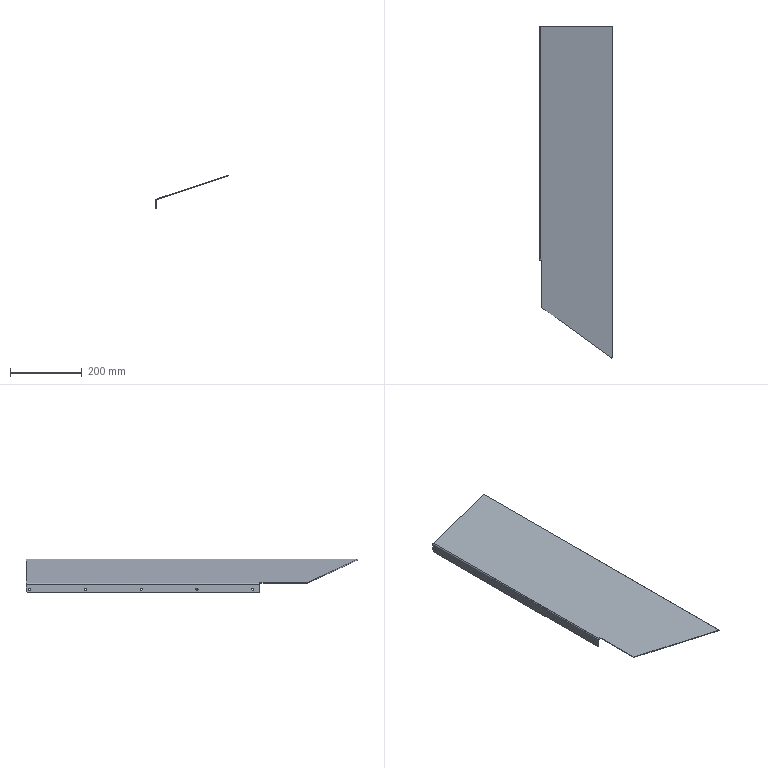Part | NX | features solid 2 | 1 solid | 25 faces | box 203 x 924.5 x 93.897 mm | volume 393378 mm3 | cylinder 14 | plane 11 | commonest cylinder face diameters 6 x10 4 x2 8 x1 20 x1
STEP:
#1=CARTESIAN_POINT('',(2192.368,-654.75,255.897));
#2=VERTEX_POINT('',#1);
#3=CARTESIAN_POINT('',(2190.47,-652.75,255.265));
#4=VERTEX_POINT('',#3);
#5=CARTESIAN_POINT('',(2190.47,-654.75,255.265));
#6=DIRECTION('',(-0.3162,0.,0.9487));
#7=DIRECTION('',(-0.9487,0.,-0.3162));
#8=AXIS2_PLACEMENT_3D('',#5,#6,#7);
#9=CIRCLE('',#8,2.);
#10=EDGE_CURVE('',#2,#4,#9,.T.);
#11=ORIENTED_EDGE('',*,*,#10,.F.);
#12=CARTESIAN_POINT('',(2193.,-654.75,254.));
#13=VERTEX_POINT('',#12);
#14=CARTESIAN_POINT('',(2193.,-654.75,254.));
#15=DIRECTION('',(-0.3162,0.,0.9487));
#16=VECTOR('',#15,1000.);
#17=LINE('',#14,#16);
#18=EDGE_CURVE('',#13,#2,#17,.T.);
#19=ORIENTED_EDGE('',*,*,#18,.F.);
#20=CARTESIAN_POINT('',(2191.103,-652.75,253.368));
#21=VERTEX_POINT('',#20);
#22=CARTESIAN_POINT('',(2191.103,-654.75,253.368));
#23=DIRECTION('',(0.3162,0.,-0.9487));
#24=DIRECTION('',(-0.9487,0.,-0.3162));
#25=AXIS2_PLACEMENT_3D('',#22,#23,#24);
#26=CIRCLE('',#25,2.);
#27=EDGE_CURVE('',#21,#13,#26,.T.);
#28=ORIENTED_EDGE('',*,*,#27,.F.);
#29=CARTESIAN_POINT('',(2191.735,-652.75,251.47));
#30=DIRECTION('',(0.3162,0.,-0.9487));
#31=VECTOR('',#30,1000.);
#32=LINE('',#29,#31);
#33=EDGE_CURVE('',#4,#21,#32,.T.);
#34=ORIENTED_EDGE('',*,*,#33,.F.);
#35=EDGE_LOOP('',(#11,#19,#28,#34));
#36=FACE_BOUND('',#35,.T.);
#37=CARTESIAN_POINT('',(2191.735,-654.75,251.47));
#38=DIRECTION('',(0.3162,0.,-0.9487));
#39=DIRECTION('',(0.9487,0.,0.3162));
#40=AXIS2_PLACEMENT_3D('',#37,#38,#39);
#41=CYLINDRICAL_SURFACE('',#40,2.);
#42=ADVANCED_FACE('',(#36),#41,.T.);
#43=CARTESIAN_POINT('',(1990.,-652.75,172.));
#44=VERTEX_POINT('',#43);
#45=CARTESIAN_POINT('',(1990.,-662.75,162.));
#46=VERTEX_POINT('',#45);
#47=CARTESIAN_POINT('',(1990.,-662.75,172.));
#48=DIRECTION('',(-1.,0.,0.));
#49=DIRECTION('',(0.,0.,-1.));
#50=AXIS2_PLACEMENT_3D('',#47,#48,#49);
#51=CIRCLE('',#50,10.);
#52=EDGE_CURVE('',#44,#46,#51,.T.);
#53=ORIENTED_EDGE('',*,*,#52,.F.);
#54=CARTESIAN_POINT('',(1992.,-652.75,172.));
#55=VERTEX_POINT('',#54);
#56=CARTESIAN_POINT('',(1994.,-652.75,172.));
#57=DIRECTION('',(-1.,0.,0.));
#58=VECTOR('',#57,1000.);
#59=LINE('',#56,#58);
#60=EDGE_CURVE('',#55,#44,#59,.T.);
#61=ORIENTED_EDGE('',*,*,#60,.F.);
#62=CARTESIAN_POINT('',(1992.,-662.75,162.));
#63=VERTEX_POINT('',#62);
#64=CARTESIAN_POINT('',(1992.,-662.75,172.));
#65=DIRECTION('',(1.,0.,0.));
#66=DIRECTION('',(0.,0.,-1.));
#67=AXIS2_PLACEMENT_3D('',#64,#65,#66);
#68=CIRCLE('',#67,10.);
#69=EDGE_CURVE('',#63,#55,#68,.T.);
#70=ORIENTED_EDGE('',*,*,#69,.F.);
#71=CARTESIAN_POINT('',(1992.,-662.75,162.));
#72=DIRECTION('',(1.,0.,0.));
#73=VECTOR('',#72,1000.);
#74=LINE('',#71,#73);
#75=EDGE_CURVE('',#46,#63,#74,.T.);
#76=ORIENTED_EDGE('',*,*,#75,.F.);
#77=EDGE_LOOP('',(#53,#61,#70,#76));
#78=FACE_BOUND('',#77,.T.);
#79=CARTESIAN_POINT('',(1992.,-662.75,172.));
#80=DIRECTION('',(-1.,0.,0.));
#81=DIRECTION('',(0.,-1.,0.));
#82=AXIS2_PLACEMENT_3D('',#79,#80,#81);
#83=CYLINDRICAL_SURFACE('',#82,10.);
#84=ADVANCED_FACE('',(#78),#83,.T.);
#85=CARTESIAN_POINT('',(1992.,-1284.25,175.));
#86=VERTEX_POINT('',#85);
#87=CARTESIAN_POINT('',(1990.,-1284.25,175.));
#88=VERTEX_POINT('',#87);
#89=CARTESIAN_POINT('',(2941.171,-1284.25,175.));
#90=DIRECTION('',(-1.,0.,0.));
#91=VECTOR('',#90,1000.);
#92=LINE('',#89,#91);
#93=EDGE_CURVE('',#86,#88,#92,.T.);
#94=ORIENTED_EDGE('',*,*,#93,.F.);
#95=CARTESIAN_POINT('',(1992.,-1284.25,169.));
#96=VERTEX_POINT('',#95);
#97=CARTESIAN_POINT('',(1992.,-1284.25,172.));
#98=DIRECTION('',(-1.,0.,0.));
#99=DIRECTION('',(0.,0.,-1.));
#100=AXIS2_PLACEMENT_3D('',#97,#98,#99);
#101=CIRCLE('',#100,3.);
#102=EDGE_CURVE('',#96,#86,#101,.T.);
#103=ORIENTED_EDGE('',*,*,#102,.F.);
#104=CARTESIAN_POINT('',(1990.,-1284.25,169.));
#105=VERTEX_POINT('',#104);
#106=CARTESIAN_POINT('',(2941.171,-1284.25,169.));
#107=DIRECTION('',(-1.,0.,0.));
#108=VECTOR('',#107,1000.);
#109=LINE('',#106,#108);
#110=EDGE_CURVE('',#105,#96,#109,.F.);
#111=ORIENTED_EDGE('',*,*,#110,.F.);
#112=CARTESIAN_POINT('',(1990.,-1284.25,172.));
#113=DIRECTION('',(-1.,0.,0.));
#114=DIRECTION('',(0.,-1.,0.));
#115=AXIS2_PLACEMENT_3D('',#112,#113,#114);
#116=CIRCLE('',#115,3.);
#117=EDGE_CURVE('',#105,#88,#116,.T.);
#118=ORIENTED_EDGE('',*,*,#117,.T.);
#119=EDGE_LOOP('',(#94,#103,#111,#118));
#120=FACE_BOUND('',#119,.T.);
#121=CARTESIAN_POINT('',(2941.171,-1284.25,172.));
#122=DIRECTION('',(-1.,0.,0.));
#123=DIRECTION('',(0.,0.,-1.));
#124=AXIS2_PLACEMENT_3D('',#121,#122,#123);
#125=CYLINDRICAL_SURFACE('',#124,3.);
#126=ADVANCED_FACE('',(#120),#125,.F.);
#127=CARTESIAN_POINT('',(1990.,-1128.875,175.));
#128=VERTEX_POINT('',#127);
#129=CARTESIAN_POINT('',(1992.,-1128.875,175.));
#130=VERTEX_POINT('',#129);
#131=CARTESIAN_POINT('',(2941.171,-1128.875,175.));
#132=DIRECTION('',(-1.,0.,0.));
#133=VECTOR('',#132,1000.);
#134=LINE('',#131,#133);
#135=EDGE_CURVE('',#128,#130,#134,.F.);
#136=ORIENTED_EDGE('',*,*,#135,.T.);
#137=CARTESIAN_POINT('',(1992.,-1128.875,169.));
#138=VERTEX_POINT('',#137);
#139=CARTESIAN_POINT('',(1992.,-1128.875,172.));
#140=DIRECTION('',(-1.,0.,0.));
#141=DIRECTION('',(0.,0.,-1.));
#142=AXIS2_PLACEMENT_3D('',#139,#140,#141);
#143=CIRCLE('',#142,3.);
#144=EDGE_CURVE('',#138,#130,#143,.T.);
#145=ORIENTED_EDGE('',*,*,#144,.F.);
#146=CARTESIAN_POINT('',(1990.,-1128.875,169.));
#147=VERTEX_POINT('',#146);
#148=CARTESIAN_POINT('',(2941.171,-1128.875,169.));
#149=DIRECTION('',(-1.,0.,0.));
#150=VECTOR('',#149,1000.);
#151=LINE('',#148,#150);
#152=EDGE_CURVE('',#138,#147,#151,.T.);
#153=ORIENTED_EDGE('',*,*,#152,.T.);
#154=CARTESIAN_POINT('',(1990.,-1128.875,172.));
#155=DIRECTION('',(-1.,0.,0.));
#156=DIRECTION('',(0.,-1.,0.));
#157=AXIS2_PLACEMENT_3D('',#154,#155,#156);
#158=CIRCLE('',#157,3.);
#159=EDGE_CURVE('',#147,#128,#158,.T.);
#160=ORIENTED_EDGE('',*,*,#159,.T.);
#161=EDGE_LOOP('',(#136,#145,#153,#160));
#162=FACE_BOUND('',#161,.T.);
#163=CARTESIAN_POINT('',(2941.171,-1128.875,172.));
#164=DIRECTION('',(-1.,0.,0.));
#165=DIRECTION('',(0.,0.,-1.));
#166=AXIS2_PLACEMENT_3D('',#163,#164,#165);
#167=CYLINDRICAL_SURFACE('',#166,3.);
#168=ADVANCED_FACE('',(#162),#167,.F.);
#169=CARTESIAN_POINT('',(1992.,-973.5,175.));
#170=VERTEX_POINT('',#169);
#171=CARTESIAN_POINT('',(1990.,-973.5,175.));
#172=VERTEX_POINT('',#171);
#173=CARTESIAN_POINT('',(2941.171,-973.5,175.));
#174=DIRECTION('',(-1.,0.,0.));
#175=VECTOR('',#174,1000.);
#176=LINE('',#173,#175);
#177=EDGE_CURVE('',#170,#172,#176,.T.);
#178=ORIENTED_EDGE('',*,*,#177,.F.);
#179=CARTESIAN_POINT('',(1992.,-973.5,169.));
#180=VERTEX_POINT('',#179);
#181=CARTESIAN_POINT('',(1992.,-973.5,172.));
#182=DIRECTION('',(-1.,0.,0.));
#183=DIRECTION('',(0.,0.,-1.));
#184=AXIS2_PLACEMENT_3D('',#181,#182,#183);
#185=CIRCLE('',#184,3.);
#186=EDGE_CURVE('',#180,#170,#185,.T.);
#187=ORIENTED_EDGE('',*,*,#186,.F.);
#188=CARTESIAN_POINT('',(1990.,-973.5,169.));
#189=VERTEX_POINT('',#188);
#190=CARTESIAN_POINT('',(2941.171,-973.5,169.));
#191=DIRECTION('',(-1.,0.,0.));
#192=VECTOR('',#191,1000.);
#193=LINE('',#190,#192);
#194=EDGE_CURVE('',#189,#180,#193,.F.);
#195=ORIENTED_EDGE('',*,*,#194,.F.);
#196=CARTESIAN_POINT('',(1990.,-973.5,172.));
#197=DIRECTION('',(-1.,0.,0.));
#198=DIRECTION('',(0.,-1.,0.));
#199=AXIS2_PLACEMENT_3D('',#196,#197,#198);
#200=CIRCLE('',#199,3.);
#201=EDGE_CURVE('',#189,#172,#200,.T.);
#202=ORIENTED_EDGE('',*,*,#201,.T.);
#203=EDGE_LOOP('',(#178,#187,#195,#202));
#204=FACE_BOUND('',#203,.T.);
#205=CARTESIAN_POINT('',(2941.171,-973.5,172.));
#206=DIRECTION('',(-1.,0.,0.));
#207=DIRECTION('',(0.,0.,-1.));
#208=AXIS2_PLACEMENT_3D('',#205,#206,#207);
#209=CYLINDRICAL_SURFACE('',#208,3.);
#210=ADVANCED_FACE('',(#204),#209,.F.);
#211=CARTESIAN_POINT('',(1992.,-818.125,175.));
#212=VERTEX_POINT('',#211);
#213=CARTESIAN_POINT('',(1990.,-818.125,175.));
#214=VERTEX_POINT('',#213);
#215=CARTESIAN_POINT('',(2941.171,-818.125,175.));
#216=DIRECTION('',(-1.,0.,0.));
#217=VECTOR('',#216,1000.);
#218=LINE('',#215,#217);
#219=EDGE_CURVE('',#212,#214,#218,.T.);
#220=ORIENTED_EDGE('',*,*,#219,.F.);
#221=CARTESIAN_POINT('',(1992.,-818.125,169.));
#222=VERTEX_POINT('',#221);
#223=CARTESIAN_POINT('',(1992.,-818.125,172.));
#224=DIRECTION('',(-1.,0.,0.));
#225=DIRECTION('',(0.,0.,-1.));
#226=AXIS2_PLACEMENT_3D('',#223,#224,#225);
#227=CIRCLE('',#226,3.);
#228=EDGE_CURVE('',#222,#212,#227,.T.);
#229=ORIENTED_EDGE('',*,*,#228,.F.);
#230=CARTESIAN_POINT('',(1990.,-818.125,169.));
#231=VERTEX_POINT('',#230);
#232=CARTESIAN_POINT('',(2941.171,-818.125,169.));
#233=DIRECTION('',(-1.,0.,0.));
#234=VECTOR('',#233,1000.);
#235=LINE('',#232,#234);
#236=EDGE_CURVE('',#231,#222,#235,.F.);
#237=ORIENTED_EDGE('',*,*,#236,.F.);
#238=CARTESIAN_POINT('',(1990.,-818.125,172.));
#239=DIRECTION('',(-1.,0.,0.));
#240=DIRECTION('',(0.,-1.,0.));
#241=AXIS2_PLACEMENT_3D('',#238,#239,#240);
#242=CIRCLE('',#241,3.);
#243=EDGE_CURVE('',#231,#214,#242,.T.);
#244=ORIENTED_EDGE('',*,*,#243,.T.);
#245=EDGE_LOOP('',(#220,#229,#237,#244));
#246=FACE_BOUND('',#245,.T.);
#247=CARTESIAN_POINT('',(2941.171,-818.125,172.));
#248=DIRECTION('',(-1.,0.,0.));
#249=DIRECTION('',(0.,0.,-1.));
#250=AXIS2_PLACEMENT_3D('',#247,#248,#249);
#251=CYLINDRICAL_SURFACE('',#250,3.);
#252=ADVANCED_FACE('',(#246),#251,.F.);
#253=CARTESIAN_POINT('',(1992.,-662.75,175.));
#254=VERTEX_POINT('',#253);
#255=CARTESIAN_POINT('',(1990.,-662.75,175.));
#256=VERTEX_POINT('',#255);
#257=CARTESIAN_POINT('',(2941.171,-662.75,175.));
#258=DIRECTION('',(-1.,0.,0.));
#259=VECTOR('',#258,1000.);
#260=LINE('',#257,#259);
#261=EDGE_CURVE('',#254,#256,#260,.T.);
#262=ORIENTED_EDGE('',*,*,#261,.F.);
#263=CARTESIAN_POINT('',(1992.,-662.75,169.));
#264=VERTEX_POINT('',#263);
#265=CARTESIAN_POINT('',(1992.,-662.75,172.));
#266=DIRECTION('',(-1.,0.,0.));
#267=DIRECTION('',(0.,0.,-1.));
#268=AXIS2_PLACEMENT_3D('',#265,#266,#267);
#269=CIRCLE('',#268,3.);
#270=EDGE_CURVE('',#264,#254,#269,.T.);
#271=ORIENTED_EDGE('',*,*,#270,.F.);
#272=CARTESIAN_POINT('',(1990.,-662.75,169.));
#273=VERTEX_POINT('',#272);
#274=CARTESIAN_POINT('',(2941.171,-662.75,169.));
#275=DIRECTION('',(-1.,0.,0.));
#276=VECTOR('',#275,1000.);
#277=LINE('',#274,#276);
#278=EDGE_CURVE('',#273,#264,#277,.F.);
#279=ORIENTED_EDGE('',*,*,#278,.F.);
#280=CARTESIAN_POINT('',(1990.,-662.75,172.));
#281=DIRECTION('',(-1.,0.,0.));
#282=DIRECTION('',(0.,-1.,0.));
#283=AXIS2_PLACEMENT_3D('',#280,#281,#282);
#284=CIRCLE('',#283,3.);
#285=EDGE_CURVE('',#273,#256,#284,.T.);
#286=ORIENTED_EDGE('',*,*,#285,.T.);
#287=EDGE_LOOP('',(#262,#271,#279,#286));
#288=FACE_BOUND('',#287,.T.);
#289=CARTESIAN_POINT('',(2941.171,-662.75,172.));
#290=DIRECTION('',(-1.,0.,0.));
#291=DIRECTION('',(0.,0.,-1.));
#292=AXIS2_PLACEMENT_3D('',#289,#290,#291);
#293=CYLINDRICAL_SURFACE('',#292,3.);
#294=ADVANCED_FACE('',(#288),#293,.F.);
#295=CARTESIAN_POINT('',(1996.725,-1304.25,190.683));
#296=VERTEX_POINT('',#295);
#297=CARTESIAN_POINT('',(1992.735,-1304.25,189.353));
#298=VERTEX_POINT('',#297);
#299=CARTESIAN_POINT('',(1991.368,-1304.25,188.897));
#300=DIRECTION('',(-0.9487,0.,-0.3162));
#301=VECTOR('',#300,1000.);
#302=LINE('',#299,#301);
#303=EDGE_CURVE('',#296,#298,#302,.T.);
#304=ORIENTED_EDGE('',*,*,#303,.T.);
#305=CARTESIAN_POINT('',(1990.,-1304.25,185.558));
#306=VERTEX_POINT('',#305);
#307=CARTESIAN_POINT('',(1994.,-1304.25,185.558));
#308=DIRECTION('',(0.,-1.,0.));
#309=DIRECTION('',(0.,0.,1.));
#310=AXIS2_PLACEMENT_3D('',#307,#308,#309);
#311=CIRCLE('',#310,4.);
#312=EDGE_CURVE('',#298,#306,#311,.T.);
#313=ORIENTED_EDGE('',*,*,#312,.T.);
#314=CARTESIAN_POINT('',(1990.,-1304.25,162.));
#315=VERTEX_POINT('',#314);
#316=CARTESIAN_POINT('',(1990.,-1304.25,162.));
#317=DIRECTION('',(0.,0.,-1.));
#318=VECTOR('',#317,1000.);
#319=LINE('',#316,#318);
#320=EDGE_CURVE('',#306,#315,#319,.T.);
#321=ORIENTED_EDGE('',*,*,#320,.T.);
#322=CARTESIAN_POINT('',(1992.,-1304.25,162.));
#323=VERTEX_POINT('',#322);
#324=CARTESIAN_POINT('',(1992.,-1304.25,162.));
#325=DIRECTION('',(1.,0.,0.));
#326=VECTOR('',#325,1000.);
#327=LINE('',#324,#326);
#328=EDGE_CURVE('',#315,#323,#327,.T.);
#329=ORIENTED_EDGE('',*,*,#328,.T.);
#330=CARTESIAN_POINT('',(1992.,-1304.25,185.558));
#331=VERTEX_POINT('',#330);
#332=CARTESIAN_POINT('',(1992.,-1304.25,162.));
#333=DIRECTION('',(0.,0.,-1.));
#334=VECTOR('',#333,1000.);
#335=LINE('',#332,#334);
#336=EDGE_CURVE('',#331,#323,#335,.T.);
#337=ORIENTED_EDGE('',*,*,#336,.F.);
#338=CARTESIAN_POINT('',(1993.368,-1304.25,187.456));
#339=VERTEX_POINT('',#338);
#340=CARTESIAN_POINT('',(1994.,-1304.25,185.558));
#341=DIRECTION('',(0.,-1.,0.));
#342=DIRECTION('',(-1.,0.,0.));
#343=AXIS2_PLACEMENT_3D('',#340,#341,#342);
#344=CIRCLE('',#343,2.);
#345=EDGE_CURVE('',#339,#331,#344,.T.);
#346=ORIENTED_EDGE('',*,*,#345,.F.);
#347=CARTESIAN_POINT('',(1997.357,-1304.25,188.786));
#348=VERTEX_POINT('',#347);
#349=CARTESIAN_POINT('',(1992.,-1304.25,187.));
#350=DIRECTION('',(-0.9487,0.,-0.3162));
#351=VECTOR('',#350,1000.);
#352=LINE('',#349,#351);
#353=EDGE_CURVE('',#348,#339,#352,.T.);
#354=ORIENTED_EDGE('',*,*,#353,.F.);
#355=CARTESIAN_POINT('',(1997.357,-1304.25,188.786));
#356=DIRECTION('',(0.3162,0.,-0.9487));
#357=VECTOR('',#356,1000.);
#358=LINE('',#355,#357);
#359=EDGE_CURVE('',#296,#348,#358,.T.);
#360=ORIENTED_EDGE('',*,*,#359,.F.);
#361=EDGE_LOOP('',(#304,#313,#321,#329,#337,#346,#354,#360));
#362=FACE_BOUND('',#361,.T.);
#363=CARTESIAN_POINT('',(1992.,-1304.25,187.));
#364=DIRECTION('',(0.,1.,0.));
#365=DIRECTION('',(0.,0.,-1.));
#366=AXIS2_PLACEMENT_3D('',#363,#364,#365);
#367=PLANE('',#366);
#368=ADVANCED_FACE('',(#362),#367,.F.);
#369=CARTESIAN_POINT('',(1996.725,-1436.889,190.683));
#370=VERTEX_POINT('',#369);
#371=CARTESIAN_POINT('',(1997.357,-1436.889,188.786));
#372=VERTEX_POINT('',#371);
#373=CARTESIAN_POINT('',(1997.357,-1436.889,188.786));
#374=DIRECTION('',(0.3162,0.,-0.9487));
#375=VECTOR('',#374,1000.);
#376=LINE('',#373,#375);
#377=EDGE_CURVE('',#370,#372,#376,.T.);
#378=ORIENTED_EDGE('',*,*,#377,.T.);
#379=CARTESIAN_POINT('',(2191.103,-1577.25,253.368));
#380=VERTEX_POINT('',#379);
#381=CARTESIAN_POINT('',(2055.875,-1479.284,208.292));
#382=DIRECTION('',(-0.7818,0.5664,-0.2606));
#383=VECTOR('',#382,1000.);
#384=LINE('',#381,#383);
#385=EDGE_CURVE('',#380,#372,#384,.T.);
#386=ORIENTED_EDGE('',*,*,#385,.F.);
#387=CARTESIAN_POINT('',(2190.47,-1577.25,255.265));
#388=VERTEX_POINT('',#387);
#389=CARTESIAN_POINT('',(2191.103,-1577.25,253.368));
#390=DIRECTION('',(0.3162,0.,-0.9487));
#391=VECTOR('',#390,1000.);
#392=LINE('',#389,#391);
#393=EDGE_CURVE('',#388,#380,#392,.T.);
#394=ORIENTED_EDGE('',*,*,#393,.F.);
#395=CARTESIAN_POINT('',(2055.243,-1479.284,210.189));
#396=DIRECTION('',(-0.7818,0.5664,-0.2606));
#397=VECTOR('',#396,1000.);
#398=LINE('',#395,#397);
#399=EDGE_CURVE('',#388,#370,#398,.T.);
#400=ORIENTED_EDGE('',*,*,#399,.T.);
#401=EDGE_LOOP('',(#378,#386,#394,#400));
#402=FACE_BOUND('',#401,.T.);
#403=CARTESIAN_POINT('',(2055.875,-1479.284,208.292));
#404=DIRECTION('',(0.5373,0.8241,0.1791));
#405=DIRECTION('',(0.3162,0.,-0.9487));
#406=AXIS2_PLACEMENT_3D('',#403,#404,#405);
#407=PLANE('',#406);
#408=ADVANCED_FACE('',(#402),#407,.F.);
#409=ORIENTED_EDGE('',*,*,#359,.T.);
#410=CARTESIAN_POINT('',(1997.357,-1577.25,188.786));
#411=DIRECTION('',(0.,1.,0.));
#412=VECTOR('',#411,1000.);
#413=LINE('',#410,#412);
#414=EDGE_CURVE('',#372,#348,#413,.T.);
#415=ORIENTED_EDGE('',*,*,#414,.F.);
#416=ORIENTED_EDGE('',*,*,#377,.F.);
#417=CARTESIAN_POINT('',(1996.725,-1577.25,190.683));
#418=DIRECTION('',(0.,1.,0.));
#419=VECTOR('',#418,1000.);
#420=LINE('',#417,#419);
#421=EDGE_CURVE('',#370,#296,#420,.T.);
#422=ORIENTED_EDGE('',*,*,#421,.T.);
#423=EDGE_LOOP('',(#409,#415,#416,#422));
#424=FACE_BOUND('',#423,.T.);
#425=CARTESIAN_POINT('',(1997.357,-1577.25,188.786));
#426=DIRECTION('',(0.9487,0.,0.3162));
#427=DIRECTION('',(0.,-1.,0.));
#428=AXIS2_PLACEMENT_3D('',#425,#426,#427);
#429=PLANE('',#428);
#430=ADVANCED_FACE('',(#424),#429,.F.);
#431=CARTESIAN_POINT('',(2192.368,-1577.25,255.897));
#432=VERTEX_POINT('',#431);
#433=CARTESIAN_POINT('',(2192.368,-1577.25,255.897));
#434=DIRECTION('',(0.,1.,0.));
#435=VECTOR('',#434,1000.);
#436=LINE('',#433,#435);
#437=EDGE_CURVE('',#432,#2,#436,.T.);
#438=ORIENTED_EDGE('',*,*,#437,.T.);
#439=ORIENTED_EDGE('',*,*,#10,.T.);
#440=CARTESIAN_POINT('',(1992.735,-652.75,189.353));
#441=VERTEX_POINT('',#440);
#442=CARTESIAN_POINT('',(1991.368,-652.75,188.897));
#443=DIRECTION('',(0.9487,0.,0.3162));
#444=VECTOR('',#443,1000.);
#445=LINE('',#442,#444);
#446=EDGE_CURVE('',#441,#4,#445,.T.);
#447=ORIENTED_EDGE('',*,*,#446,.F.);
#448=CARTESIAN_POINT('',(1992.735,-1577.25,189.353));
#449=DIRECTION('',(0.,1.,0.));
#450=VECTOR('',#449,1000.);
#451=LINE('',#448,#450);
#452=EDGE_CURVE('',#298,#441,#451,.T.);
#453=ORIENTED_EDGE('',*,*,#452,.F.);
#454=ORIENTED_EDGE('',*,*,#303,.F.);
#455=ORIENTED_EDGE('',*,*,#421,.F.);
#456=ORIENTED_EDGE('',*,*,#399,.F.);
#457=CARTESIAN_POINT('',(1991.368,-1577.25,188.897));
#458=DIRECTION('',(0.9487,0.,0.3162));
#459=VECTOR('',#458,1000.);
#460=LINE('',#457,#459);
#461=EDGE_CURVE('',#388,#432,#460,.T.);
#462=ORIENTED_EDGE('',*,*,#461,.T.);
#463=EDGE_LOOP('',(#438,#439,#447,#453,#454,#455,#456,#462));
#464=FACE_BOUND('',#463,.T.);
#465=CARTESIAN_POINT('',(1991.368,-1577.25,188.897));
#466=DIRECTION('',(-0.3162,0.,0.9487));
#467=DIRECTION('',(0.,1.,0.));
#468=AXIS2_PLACEMENT_3D('',#465,#466,#467);
#469=PLANE('',#468);
#470=ADVANCED_FACE('',(#464),#469,.T.);
#471=ORIENTED_EDGE('',*,*,#312,.F.);
#472=ORIENTED_EDGE('',*,*,#452,.T.);
#473=CARTESIAN_POINT('',(1990.,-652.75,185.558));
#474=VERTEX_POINT('',#473);
#475=CARTESIAN_POINT('',(1994.,-652.75,185.558));
#476=DIRECTION('',(0.,1.,0.));
#477=DIRECTION('',(0.,0.,1.));
#478=AXIS2_PLACEMENT_3D('',#475,#476,#477);
#479=CIRCLE('',#478,4.);
#480=EDGE_CURVE('',#474,#441,#479,.T.);
#481=ORIENTED_EDGE('',*,*,#480,.F.);
#482=CARTESIAN_POINT('',(1990.,-1577.25,185.558));
#483=DIRECTION('',(0.,1.,0.));
#484=VECTOR('',#483,1000.);
#485=LINE('',#482,#484);
#486=EDGE_CURVE('',#306,#474,#485,.T.);
#487=ORIENTED_EDGE('',*,*,#486,.F.);
#488=EDGE_LOOP('',(#471,#472,#481,#487));
#489=FACE_BOUND('',#488,.T.);
#490=CARTESIAN_POINT('',(1994.,-1577.25,185.558));
#491=DIRECTION('',(0.,1.,0.));
#492=DIRECTION('',(0.,0.,1.));
#493=AXIS2_PLACEMENT_3D('',#490,#491,#492);
#494=CYLINDRICAL_SURFACE('',#493,4.);
#495=ADVANCED_FACE('',(#489),#494,.T.);
#496=ORIENTED_EDGE('',*,*,#285,.F.);
#497=CARTESIAN_POINT('',(1990.,-662.75,172.));
#498=DIRECTION('',(-1.,0.,0.));
#499=DIRECTION('',(0.,-1.,0.));
#500=AXIS2_PLACEMENT_3D('',#497,#498,#499);
#501=CIRCLE('',#500,3.);
#502=EDGE_CURVE('',#256,#273,#501,.T.);
#503=ORIENTED_EDGE('',*,*,#502,.F.);
#504=EDGE_LOOP('',(#496,#503));
#505=FACE_BOUND('',#504,.T.);
#506=ORIENTED_EDGE('',*,*,#243,.F.);
#507=CARTESIAN_POINT('',(1990.,-818.125,172.));
#508=DIRECTION('',(-1.,0.,0.));
#509=DIRECTION('',(0.,-1.,0.));
#510=AXIS2_PLACEMENT_3D('',#507,#508,#509);
#511=CIRCLE('',#510,3.);
#512=EDGE_CURVE('',#214,#231,#511,.T.);
#513=ORIENTED_EDGE('',*,*,#512,.F.);
#514=EDGE_LOOP('',(#506,#513));
#515=FACE_BOUND('',#514,.T.);
#516=ORIENTED_EDGE('',*,*,#201,.F.);
#517=CARTESIAN_POINT('',(1990.,-973.5,172.));
#518=DIRECTION('',(-1.,0.,0.));
#519=DIRECTION('',(0.,-1.,0.));
#520=AXIS2_PLACEMENT_3D('',#517,#518,#519);
#521=CIRCLE('',#520,3.);
#522=EDGE_CURVE('',#172,#189,#521,.T.);
#523=ORIENTED_EDGE('',*,*,#522,.F.);
#524=EDGE_LOOP('',(#516,#523));
#525=FACE_BOUND('',#524,.T.);
#526=ORIENTED_EDGE('',*,*,#159,.F.);
#527=CARTESIAN_POINT('',(1990.,-1128.875,172.));
#528=DIRECTION('',(-1.,0.,0.));
#529=DIRECTION('',(0.,-1.,0.));
#530=AXIS2_PLACEMENT_3D('',#527,#528,#529);
#531=CIRCLE('',#530,3.);
#532=EDGE_CURVE('',#128,#147,#531,.T.);
#533=ORIENTED_EDGE('',*,*,#532,.F.);
#534=EDGE_LOOP('',(#526,#533));
#535=FACE_BOUND('',#534,.T.);
#536=ORIENTED_EDGE('',*,*,#117,.F.);
#537=CARTESIAN_POINT('',(1990.,-1284.25,172.));
#538=DIRECTION('',(-1.,0.,0.));
#539=DIRECTION('',(0.,-1.,0.));
#540=AXIS2_PLACEMENT_3D('',#537,#538,#539);
#541=CIRCLE('',#540,3.);
#542=EDGE_CURVE('',#88,#105,#541,.T.);
#543=ORIENTED_EDGE('',*,*,#542,.F.);
#544=EDGE_LOOP('',(#536,#543));
#545=FACE_BOUND('',#544,.T.);
#546=CARTESIAN_POINT('',(1990.,-652.75,162.));
#547=DIRECTION('',(0.,0.,1.));
#548=VECTOR('',#547,1000.);
#549=LINE('',#546,#548);
#550=EDGE_CURVE('',#44,#474,#549,.T.);
#551=ORIENTED_EDGE('',*,*,#550,.F.);
#552=ORIENTED_EDGE('',*,*,#52,.T.);
#553=CARTESIAN_POINT('',(1990.,-1577.25,162.));
#554=DIRECTION('',(0.,1.,0.));
#555=VECTOR('',#554,1000.);
#556=LINE('',#553,#555);
#557=EDGE_CURVE('',#315,#46,#556,.T.);
#558=ORIENTED_EDGE('',*,*,#557,.F.);
#559=ORIENTED_EDGE('',*,*,#320,.F.);
#560=ORIENTED_EDGE('',*,*,#486,.T.);
#561=EDGE_LOOP('',(#551,#552,#558,#559,#560));
#562=FACE_BOUND('',#561,.T.);
#563=CARTESIAN_POINT('',(1990.,-1577.25,162.));
#564=DIRECTION('',(-1.,0.,0.));
#565=DIRECTION('',(0.,0.,1.));
#566=AXIS2_PLACEMENT_3D('',#563,#564,#565);
#567=PLANE('',#566);
#568=ADVANCED_FACE('',(#505,#515,#525,#535,#545,#562),#567,.T.);
#569=CARTESIAN_POINT('',(1993.368,-652.75,187.456));
#570=VERTEX_POINT('',#569);
#571=CARTESIAN_POINT('',(1992.,-652.75,187.));
#572=DIRECTION('',(0.9487,0.,0.3162));
#573=VECTOR('',#572,1000.);
#574=LINE('',#571,#573);
#575=EDGE_CURVE('',#570,#21,#574,.T.);
#576=ORIENTED_EDGE('',*,*,#575,.T.);
#577=ORIENTED_EDGE('',*,*,#27,.T.);
#578=CARTESIAN_POINT('',(2193.,-1577.25,254.));
#579=VERTEX_POINT('',#578);
#580=CARTESIAN_POINT('',(2193.,-1577.25,254.));
#581=DIRECTION('',(0.,1.,0.));
#582=VECTOR('',#581,1000.);
#583=LINE('',#580,#582);
#584=EDGE_CURVE('',#579,#13,#583,.T.);
#585=ORIENTED_EDGE('',*,*,#584,.F.);
#586=CARTESIAN_POINT('',(1992.,-1577.25,187.));
#587=DIRECTION('',(0.9487,0.,0.3162));
#588=VECTOR('',#587,1000.);
#589=LINE('',#586,#588);
#590=EDGE_CURVE('',#380,#579,#589,.T.);
#591=ORIENTED_EDGE('',*,*,#590,.F.);
#592=ORIENTED_EDGE('',*,*,#385,.T.);
#593=ORIENTED_EDGE('',*,*,#414,.T.);
#594=ORIENTED_EDGE('',*,*,#353,.T.);
#595=CARTESIAN_POINT('',(1993.368,-1577.25,187.456));
#596=DIRECTION('',(0.,1.,0.));
#597=VECTOR('',#596,1000.);
#598=LINE('',#595,#597);
#599=EDGE_CURVE('',#339,#570,#598,.T.);
#600=ORIENTED_EDGE('',*,*,#599,.T.);
#601=EDGE_LOOP('',(#576,#577,#585,#591,#592,#593,#594,#600));
#602=FACE_BOUND('',#601,.T.);
#603=CARTESIAN_POINT('',(1992.,-1577.25,187.));
#604=DIRECTION('',(-0.3162,0.,0.9487));
#605=DIRECTION('',(0.,1.,0.));
#606=AXIS2_PLACEMENT_3D('',#603,#604,#605);
#607=PLANE('',#606);
#608=ADVANCED_FACE('',(#602),#607,.F.);
#609=ORIENTED_EDGE('',*,*,#599,.F.);
#610=ORIENTED_EDGE('',*,*,#345,.T.);
#611=CARTESIAN_POINT('',(1992.,-652.75,185.558));
#612=VERTEX_POINT('',#611);
#613=CARTESIAN_POINT('',(1992.,-1577.25,185.558));
#614=DIRECTION('',(0.,1.,0.));
#615=VECTOR('',#614,1000.);
#616=LINE('',#613,#615);
#617=EDGE_CURVE('',#331,#612,#616,.T.);
#618=ORIENTED_EDGE('',*,*,#617,.T.);
#619=CARTESIAN_POINT('',(1994.,-652.75,185.558));
#620=DIRECTION('',(0.,1.,0.));
#621=DIRECTION('',(1.,0.,0.));
#622=AXIS2_PLACEMENT_3D('',#619,#620,#621);
#623=CIRCLE('',#622,2.);
#624=EDGE_CURVE('',#612,#570,#623,.T.);
#625=ORIENTED_EDGE('',*,*,#624,.T.);
#626=EDGE_LOOP('',(#609,#610,#618,#625));
#627=FACE_BOUND('',#626,.T.);
#628=CARTESIAN_POINT('',(1994.,-1577.25,185.558));
#629=DIRECTION('',(0.,1.,0.));
#630=DIRECTION('',(0.,0.,1.));
#631=AXIS2_PLACEMENT_3D('',#628,#629,#630);
#632=CYLINDRICAL_SURFACE('',#631,2.);
#633=ADVANCED_FACE('',(#627),#632,.F.);
#634=ORIENTED_EDGE('',*,*,#270,.T.);
#635=CARTESIAN_POINT('',(1992.,-662.75,172.));
#636=DIRECTION('',(-1.,0.,0.));
#637=DIRECTION('',(0.,0.,-1.));
#638=AXIS2_PLACEMENT_3D('',#635,#636,#637);
#639=CIRCLE('',#638,3.);
#640=EDGE_CURVE('',#254,#264,#639,.T.);
#641=ORIENTED_EDGE('',*,*,#640,.T.);
#642=EDGE_LOOP('',(#634,#641));
#643=FACE_BOUND('',#642,.T.);
#644=ORIENTED_EDGE('',*,*,#228,.T.);
#645=CARTESIAN_POINT('',(1992.,-818.125,172.));
#646=DIRECTION('',(-1.,0.,0.));
#647=DIRECTION('',(0.,0.,-1.));
#648=AXIS2_PLACEMENT_3D('',#645,#646,#647);
#649=CIRCLE('',#648,3.);
#650=EDGE_CURVE('',#212,#222,#649,.T.);
#651=ORIENTED_EDGE('',*,*,#650,.T.);
#652=EDGE_LOOP('',(#644,#651));
#653=FACE_BOUND('',#652,.T.);
#654=ORIENTED_EDGE('',*,*,#186,.T.);
#655=CARTESIAN_POINT('',(1992.,-973.5,172.));
#656=DIRECTION('',(-1.,0.,0.));
#657=DIRECTION('',(0.,0.,-1.));
#658=AXIS2_PLACEMENT_3D('',#655,#656,#657);
#659=CIRCLE('',#658,3.);
#660=EDGE_CURVE('',#170,#180,#659,.T.);
#661=ORIENTED_EDGE('',*,*,#660,.T.);
#662=EDGE_LOOP('',(#654,#661));
#663=FACE_BOUND('',#662,.T.);
#664=ORIENTED_EDGE('',*,*,#144,.T.);
#665=CARTESIAN_POINT('',(1992.,-1128.875,172.));
#666=DIRECTION('',(-1.,0.,0.));
#667=DIRECTION('',(0.,0.,-1.));
#668=AXIS2_PLACEMENT_3D('',#665,#666,#667);
#669=CIRCLE('',#668,3.);
#670=EDGE_CURVE('',#130,#138,#669,.T.);
#671=ORIENTED_EDGE('',*,*,#670,.T.);
#672=EDGE_LOOP('',(#664,#671));
#673=FACE_BOUND('',#672,.T.);
#674=ORIENTED_EDGE('',*,*,#102,.T.);
#675=CARTESIAN_POINT('',(1992.,-1284.25,172.));
#676=DIRECTION('',(-1.,0.,0.));
#677=DIRECTION('',(0.,0.,-1.));
#678=AXIS2_PLACEMENT_3D('',#675,#676,#677);
#679=CIRCLE('',#678,3.);
#680=EDGE_CURVE('',#86,#96,#679,.T.);
#681=ORIENTED_EDGE('',*,*,#680,.T.);
#682=EDGE_LOOP('',(#674,#681));
#683=FACE_BOUND('',#682,.T.);
#684=CARTESIAN_POINT('',(1992.,-1577.25,162.));
#685=DIRECTION('',(0.,1.,0.));
#686=VECTOR('',#685,1000.);
#687=LINE('',#684,#686);
#688=EDGE_CURVE('',#323,#63,#687,.T.);
#689=ORIENTED_EDGE('',*,*,#688,.T.);
#690=ORIENTED_EDGE('',*,*,#69,.T.);
#691=CARTESIAN_POINT('',(1992.,-652.75,162.));
#692=DIRECTION('',(0.,0.,1.));
#693=VECTOR('',#692,1000.);
#694=LINE('',#691,#693);
#695=EDGE_CURVE('',#55,#612,#694,.T.);
#696=ORIENTED_EDGE('',*,*,#695,.T.);
#697=ORIENTED_EDGE('',*,*,#617,.F.);
#698=ORIENTED_EDGE('',*,*,#336,.T.);
#699=EDGE_LOOP('',(#689,#690,#696,#697,#698));
#700=FACE_BOUND('',#699,.T.);
#701=CARTESIAN_POINT('',(1992.,-1577.25,162.));
#702=DIRECTION('',(-1.,0.,0.));
#703=DIRECTION('',(0.,0.,1.));
#704=AXIS2_PLACEMENT_3D('',#701,#702,#703);
#705=PLANE('',#704);
#706=ADVANCED_FACE('',(#643,#653,#663,#673,#683,#700),#705,.F.);
#707=ORIENTED_EDGE('',*,*,#446,.T.);
#708=ORIENTED_EDGE('',*,*,#33,.T.);
#709=ORIENTED_EDGE('',*,*,#575,.F.);
#710=ORIENTED_EDGE('',*,*,#624,.F.);
#711=ORIENTED_EDGE('',*,*,#695,.F.);
#712=ORIENTED_EDGE('',*,*,#60,.T.);
#713=ORIENTED_EDGE('',*,*,#550,.T.);
#714=ORIENTED_EDGE('',*,*,#480,.T.);
#715=EDGE_LOOP('',(#707,#708,#709,#710,#711,#712,#713,#714));
#716=FACE_BOUND('',#715,.T.);
#717=CARTESIAN_POINT('',(1994.,-652.75,185.558));
#718=DIRECTION('',(0.,1.,0.));
#719=DIRECTION('',(0.,0.,-1.));
#720=AXIS2_PLACEMENT_3D('',#717,#718,#719);
#721=PLANE('',#720);
#722=ADVANCED_FACE('',(#716),#721,.T.);
#723=ORIENTED_EDGE('',*,*,#557,.T.);
#724=ORIENTED_EDGE('',*,*,#75,.T.);
#725=ORIENTED_EDGE('',*,*,#688,.F.);
#726=ORIENTED_EDGE('',*,*,#328,.F.);
#727=EDGE_LOOP('',(#723,#724,#725,#726));
#728=FACE_BOUND('',#727,.T.);
#729=CARTESIAN_POINT('',(1992.,-1577.25,162.));
#730=DIRECTION('',(0.,0.,1.));
#731=DIRECTION('',(1.,0.,0.));
#732=AXIS2_PLACEMENT_3D('',#729,#730,#731);
#733=PLANE('',#732);
#734=ADVANCED_FACE('',(#728),#733,.F.);
#735=ORIENTED_EDGE('',*,*,#584,.T.);
#736=ORIENTED_EDGE('',*,*,#18,.T.);
#737=ORIENTED_EDGE('',*,*,#437,.F.);
#738=CARTESIAN_POINT('',(2193.,-1577.25,254.));
#739=DIRECTION('',(0.3162,0.,-0.9487));
#740=VECTOR('',#739,1000.);
#741=LINE('',#738,#740);
#742=EDGE_CURVE('',#432,#579,#741,.T.);
#743=ORIENTED_EDGE('',*,*,#742,.T.);
#744=EDGE_LOOP('',(#735,#736,#737,#743));
#745=FACE_BOUND('',#744,.T.);
#746=CARTESIAN_POINT('',(2193.,-1577.25,254.));
#747=DIRECTION('',(0.9487,0.,0.3162));
#748=DIRECTION('',(0.,-1.,0.));
#749=AXIS2_PLACEMENT_3D('',#746,#747,#748);
#750=PLANE('',#749);
#751=ADVANCED_FACE('',(#745),#750,.T.);
#752=ORIENTED_EDGE('',*,*,#461,.F.);
#753=ORIENTED_EDGE('',*,*,#393,.T.);
#754=ORIENTED_EDGE('',*,*,#590,.T.);
#755=ORIENTED_EDGE('',*,*,#742,.F.);
#756=EDGE_LOOP('',(#752,#753,#754,#755));
#757=FACE_BOUND('',#756,.T.);
#758=CARTESIAN_POINT('',(1992.,-1577.25,162.));
#759=DIRECTION('',(0.,-1.,0.));
#760=DIRECTION('',(-1.,0.,0.));
#761=AXIS2_PLACEMENT_3D('',#758,#759,#760);
#762=PLANE('',#761);
#763=ADVANCED_FACE('',(#757),#762,.T.);
#764=ORIENTED_EDGE('',*,*,#640,.F.);
#765=ORIENTED_EDGE('',*,*,#261,.T.);
#766=ORIENTED_EDGE('',*,*,#502,.T.);
#767=ORIENTED_EDGE('',*,*,#278,.T.);
#768=EDGE_LOOP('',(#764,#765,#766,#767));
#769=FACE_BOUND('',#768,.T.);
#770=CARTESIAN_POINT('',(2941.171,-662.75,172.));
#771=DIRECTION('',(-1.,0.,0.));
#772=DIRECTION('',(0.,0.,-1.));
#773=AXIS2_PLACEMENT_3D('',#770,#771,#772);
#774=CYLINDRICAL_SURFACE('',#773,3.);
#775=ADVANCED_FACE('',(#769),#774,.F.);
#776=ORIENTED_EDGE('',*,*,#650,.F.);
#777=ORIENTED_EDGE('',*,*,#219,.T.);
#778=ORIENTED_EDGE('',*,*,#512,.T.);
#779=ORIENTED_EDGE('',*,*,#236,.T.);
#780=EDGE_LOOP('',(#776,#777,#778,#779));
#781=FACE_BOUND('',#780,.T.);
#782=CARTESIAN_POINT('',(2941.171,-818.125,172.));
#783=DIRECTION('',(-1.,0.,0.));
#784=DIRECTION('',(0.,0.,-1.));
#785=AXIS2_PLACEMENT_3D('',#782,#783,#784);
#786=CYLINDRICAL_SURFACE('',#785,3.);
#787=ADVANCED_FACE('',(#781),#786,.F.);
#788=ORIENTED_EDGE('',*,*,#660,.F.);
#789=ORIENTED_EDGE('',*,*,#177,.T.);
#790=ORIENTED_EDGE('',*,*,#522,.T.);
#791=ORIENTED_EDGE('',*,*,#194,.T.);
#792=EDGE_LOOP('',(#788,#789,#790,#791));
#793=FACE_BOUND('',#792,.T.);
#794=CARTESIAN_POINT('',(2941.171,-973.5,172.));
#795=DIRECTION('',(-1.,0.,0.));
#796=DIRECTION('',(0.,0.,-1.));
#797=AXIS2_PLACEMENT_3D('',#794,#795,#796);
#798=CYLINDRICAL_SURFACE('',#797,3.);
#799=ADVANCED_FACE('',(#793),#798,.F.);
#800=ORIENTED_EDGE('',*,*,#670,.F.);
#801=ORIENTED_EDGE('',*,*,#135,.F.);
#802=ORIENTED_EDGE('',*,*,#532,.T.);
#803=ORIENTED_EDGE('',*,*,#152,.F.);
#804=EDGE_LOOP('',(#800,#801,#802,#803));
#805=FACE_BOUND('',#804,.T.);
#806=CARTESIAN_POINT('',(2941.171,-1128.875,172.));
#807=DIRECTION('',(-1.,0.,0.));
#808=DIRECTION('',(0.,0.,-1.));
#809=AXIS2_PLACEMENT_3D('',#806,#807,#808);
#810=CYLINDRICAL_SURFACE('',#809,3.);
#811=ADVANCED_FACE('',(#805),#810,.F.);
#812=ORIENTED_EDGE('',*,*,#680,.F.);
#813=ORIENTED_EDGE('',*,*,#93,.T.);
#814=ORIENTED_EDGE('',*,*,#542,.T.);
#815=ORIENTED_EDGE('',*,*,#110,.T.);
#816=EDGE_LOOP('',(#812,#813,#814,#815));
#817=FACE_BOUND('',#816,.T.);
#818=CARTESIAN_POINT('',(2941.171,-1284.25,172.));
#819=DIRECTION('',(-1.,0.,0.));
#820=DIRECTION('',(0.,0.,-1.));
#821=AXIS2_PLACEMENT_3D('',#818,#819,#820);
#822=CYLINDRICAL_SURFACE('',#821,3.);
#823=ADVANCED_FACE('',(#817),#822,.F.);
#824=CLOSED_SHELL('',(#42,#84,#126,#168,#210,#252,#294,#368,#408,#430,#470,#495,#568,#608,#633,#706,#722,#734,#751,#763,#775,#787,#799,#811,#823));
#825=MANIFOLD_SOLID_BREP('',#824);
#826=(LENGTH_UNIT()NAMED_UNIT(*)SI_UNIT(.MILLI.,.METRE.));
#827=UNCERTAINTY_MEASURE_WITH_UNIT(LENGTH_MEASURE(0.00001),#826,'','');
#828=(NAMED_UNIT(*)PLANE_ANGLE_UNIT()SI_UNIT($,.RADIAN.));
#829=(NAMED_UNIT(*)SI_UNIT($,.STERADIAN.)SOLID_ANGLE_UNIT());
#830=(GEOMETRIC_REPRESENTATION_CONTEXT(3)GLOBAL_UNCERTAINTY_ASSIGNED_CONTEXT((#827))GLOBAL_UNIT_ASSIGNED_CONTEXT((#826,#828,#829))REPRESENTATION_CONTEXT('',''));
#831=ADVANCED_BREP_SHAPE_REPRESENTATION('',(#825),#830);